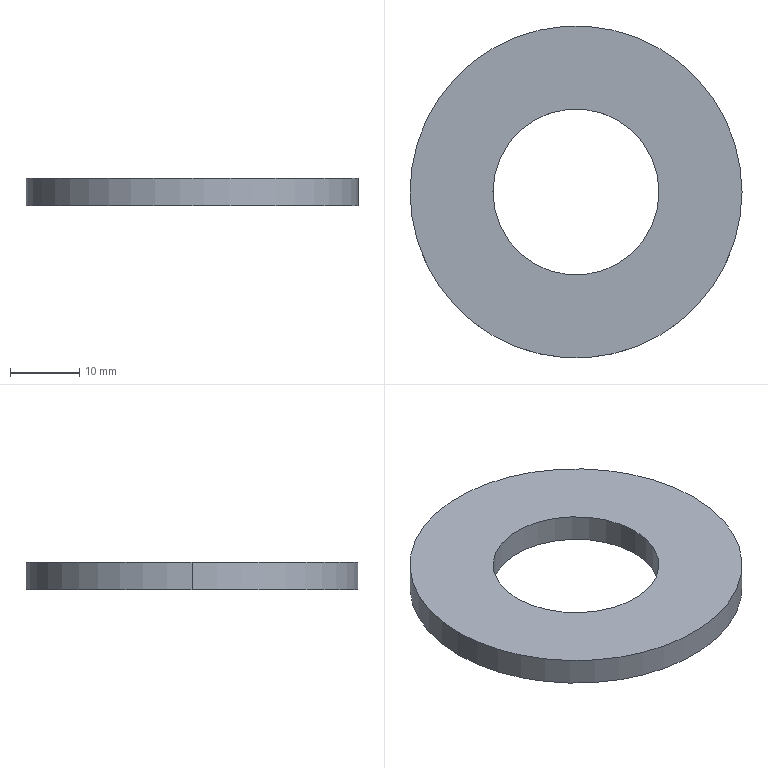Part | SolidWorks | features Extrusion 1 | 1 solid | 6 faces | box 48 x 48 x 4 mm | volume 5429 mm3 | cylinder 4 | plane 2 | commonest cylinder face diameters 24 x2 48 x2
STEP:
#1=CARTESIAN_POINT('',(-12.,0.,4.));
#2=VERTEX_POINT('',#1);
#3=CARTESIAN_POINT('',(12.,0.,4.));
#4=VERTEX_POINT('',#3);
#5=CARTESIAN_POINT('',(0.,0.,4.));
#6=DIRECTION('',(0.,0.,1.));
#7=DIRECTION('',(1.,0.,0.));
#8=AXIS2_PLACEMENT_3D('',#5,#6,#7);
#9=CIRCLE('',#8,12.);
#10=EDGE_CURVE('',#2,#4,#9,.T.);
#11=ORIENTED_EDGE('',*,*,#10,.T.);
#12=CARTESIAN_POINT('',(12.,0.,0.));
#13=VERTEX_POINT('',#12);
#14=CARTESIAN_POINT('',(12.,0.,4.));
#15=DIRECTION('',(0.,0.,-1.));
#16=VECTOR('',#15,1000.);
#17=LINE('',#14,#16);
#18=EDGE_CURVE('',#4,#13,#17,.T.);
#19=ORIENTED_EDGE('',*,*,#18,.T.);
#20=CARTESIAN_POINT('',(-12.,0.,0.));
#21=VERTEX_POINT('',#20);
#22=CARTESIAN_POINT('',(0.,0.,0.));
#23=DIRECTION('',(0.,0.,1.));
#24=DIRECTION('',(1.,0.,0.));
#25=AXIS2_PLACEMENT_3D('',#22,#23,#24);
#26=CIRCLE('',#25,12.);
#27=EDGE_CURVE('',#21,#13,#26,.T.);
#28=ORIENTED_EDGE('',*,*,#27,.F.);
#29=CARTESIAN_POINT('',(-12.,0.,4.));
#30=DIRECTION('',(0.,0.,-1.));
#31=VECTOR('',#30,1000.);
#32=LINE('',#29,#31);
#33=EDGE_CURVE('',#2,#21,#32,.T.);
#34=ORIENTED_EDGE('',*,*,#33,.F.);
#35=EDGE_LOOP('',(#11,#19,#28,#34));
#36=FACE_OUTER_BOUND('',#35,.T.);
#37=CARTESIAN_POINT('',(0.,0.,4.));
#38=DIRECTION('',(0.,0.,-1.));
#39=DIRECTION('',(-1.,0.,0.));
#40=AXIS2_PLACEMENT_3D('',#37,#38,#39);
#41=CYLINDRICAL_SURFACE('',#40,12.);
#42=ADVANCED_FACE('',(#36),#41,.F.);
#43=CARTESIAN_POINT('',(24.,0.,4.));
#44=VERTEX_POINT('',#43);
#45=CARTESIAN_POINT('',(-24.,0.,4.));
#46=VERTEX_POINT('',#45);
#47=CARTESIAN_POINT('',(0.,0.,4.));
#48=DIRECTION('',(0.,0.,1.));
#49=DIRECTION('',(1.,0.,0.));
#50=AXIS2_PLACEMENT_3D('',#47,#48,#49);
#51=CIRCLE('',#50,24.);
#52=EDGE_CURVE('',#44,#46,#51,.T.);
#53=ORIENTED_EDGE('',*,*,#52,.F.);
#54=CARTESIAN_POINT('',(24.,0.,0.));
#55=VERTEX_POINT('',#54);
#56=CARTESIAN_POINT('',(24.,0.,4.));
#57=DIRECTION('',(0.,0.,-1.));
#58=VECTOR('',#57,1000.);
#59=LINE('',#56,#58);
#60=EDGE_CURVE('',#44,#55,#59,.T.);
#61=ORIENTED_EDGE('',*,*,#60,.T.);
#62=CARTESIAN_POINT('',(-24.,0.,0.));
#63=VERTEX_POINT('',#62);
#64=CARTESIAN_POINT('',(0.,0.,0.));
#65=DIRECTION('',(0.,0.,1.));
#66=DIRECTION('',(1.,0.,0.));
#67=AXIS2_PLACEMENT_3D('',#64,#65,#66);
#68=CIRCLE('',#67,24.);
#69=EDGE_CURVE('',#55,#63,#68,.T.);
#70=ORIENTED_EDGE('',*,*,#69,.T.);
#71=CARTESIAN_POINT('',(-24.,0.,4.));
#72=DIRECTION('',(0.,0.,-1.));
#73=VECTOR('',#72,1000.);
#74=LINE('',#71,#73);
#75=EDGE_CURVE('',#46,#63,#74,.T.);
#76=ORIENTED_EDGE('',*,*,#75,.F.);
#77=EDGE_LOOP('',(#53,#61,#70,#76));
#78=FACE_OUTER_BOUND('',#77,.T.);
#79=CARTESIAN_POINT('',(0.,0.,4.));
#80=DIRECTION('',(0.,0.,-1.));
#81=DIRECTION('',(-1.,0.,0.));
#82=AXIS2_PLACEMENT_3D('',#79,#80,#81);
#83=CYLINDRICAL_SURFACE('',#82,24.);
#84=ADVANCED_FACE('',(#78),#83,.T.);
#85=CARTESIAN_POINT('',(0.,0.,4.));
#86=DIRECTION('',(0.,0.,1.));
#87=DIRECTION('',(1.,0.,0.));
#88=AXIS2_PLACEMENT_3D('',#85,#86,#87);
#89=CIRCLE('',#88,24.);
#90=EDGE_CURVE('',#46,#44,#89,.T.);
#91=ORIENTED_EDGE('',*,*,#90,.T.);
#92=ORIENTED_EDGE('',*,*,#52,.T.);
#93=EDGE_LOOP('',(#91,#92));
#94=FACE_OUTER_BOUND('',#93,.T.);
#95=ORIENTED_EDGE('',*,*,#10,.F.);
#96=CARTESIAN_POINT('',(0.,0.,4.));
#97=DIRECTION('',(0.,0.,1.));
#98=DIRECTION('',(1.,0.,0.));
#99=AXIS2_PLACEMENT_3D('',#96,#97,#98);
#100=CIRCLE('',#99,12.);
#101=EDGE_CURVE('',#4,#2,#100,.T.);
#102=ORIENTED_EDGE('',*,*,#101,.F.);
#103=EDGE_LOOP('',(#95,#102));
#104=FACE_BOUND('',#103,.T.);
#105=CARTESIAN_POINT('',(0.,0.,4.));
#106=DIRECTION('',(0.,0.,1.));
#107=DIRECTION('',(1.,0.,0.));
#108=AXIS2_PLACEMENT_3D('',#105,#106,#107);
#109=PLANE('',#108);
#110=ADVANCED_FACE('',(#94,#104),#109,.T.);
#111=CARTESIAN_POINT('',(0.,0.,0.));
#112=DIRECTION('',(0.,0.,1.));
#113=DIRECTION('',(1.,0.,0.));
#114=AXIS2_PLACEMENT_3D('',#111,#112,#113);
#115=CIRCLE('',#114,24.);
#116=EDGE_CURVE('',#63,#55,#115,.T.);
#117=ORIENTED_EDGE('',*,*,#116,.F.);
#118=ORIENTED_EDGE('',*,*,#69,.F.);
#119=EDGE_LOOP('',(#117,#118));
#120=FACE_OUTER_BOUND('',#119,.T.);
#121=ORIENTED_EDGE('',*,*,#27,.T.);
#122=CARTESIAN_POINT('',(0.,0.,0.));
#123=DIRECTION('',(0.,0.,1.));
#124=DIRECTION('',(1.,0.,0.));
#125=AXIS2_PLACEMENT_3D('',#122,#123,#124);
#126=CIRCLE('',#125,12.);
#127=EDGE_CURVE('',#13,#21,#126,.T.);
#128=ORIENTED_EDGE('',*,*,#127,.T.);
#129=EDGE_LOOP('',(#121,#128));
#130=FACE_BOUND('',#129,.T.);
#131=CARTESIAN_POINT('',(0.,0.,0.));
#132=DIRECTION('',(0.,0.,1.));
#133=DIRECTION('',(1.,0.,0.));
#134=AXIS2_PLACEMENT_3D('',#131,#132,#133);
#135=PLANE('',#134);
#136=ADVANCED_FACE('',(#120,#130),#135,.F.);
#137=ORIENTED_EDGE('',*,*,#60,.F.);
#138=ORIENTED_EDGE('',*,*,#90,.F.);
#139=ORIENTED_EDGE('',*,*,#75,.T.);
#140=ORIENTED_EDGE('',*,*,#116,.T.);
#141=EDGE_LOOP('',(#137,#138,#139,#140));
#142=FACE_OUTER_BOUND('',#141,.T.);
#143=CARTESIAN_POINT('',(0.,0.,4.));
#144=DIRECTION('',(0.,0.,-1.));
#145=DIRECTION('',(-1.,0.,0.));
#146=AXIS2_PLACEMENT_3D('',#143,#144,#145);
#147=CYLINDRICAL_SURFACE('',#146,24.);
#148=ADVANCED_FACE('',(#142),#147,.T.);
#149=ORIENTED_EDGE('',*,*,#18,.F.);
#150=ORIENTED_EDGE('',*,*,#101,.T.);
#151=ORIENTED_EDGE('',*,*,#33,.T.);
#152=ORIENTED_EDGE('',*,*,#127,.F.);
#153=EDGE_LOOP('',(#149,#150,#151,#152));
#154=FACE_OUTER_BOUND('',#153,.T.);
#155=CARTESIAN_POINT('',(0.,0.,4.));
#156=DIRECTION('',(0.,0.,-1.));
#157=DIRECTION('',(-1.,0.,0.));
#158=AXIS2_PLACEMENT_3D('',#155,#156,#157);
#159=CYLINDRICAL_SURFACE('',#158,12.);
#160=ADVANCED_FACE('',(#154),#159,.F.);
#161=CLOSED_SHELL('',(#42,#84,#110,#136,#148,#160));
#162=MANIFOLD_SOLID_BREP('',#161);
#163=CARTESIAN_POINT('',(0.,0.,0.));
#164=DIRECTION('',(0.,0.,1.));
#165=DIRECTION('',(1.,0.,0.));
#166=AXIS2_PLACEMENT_3D('',#163,#164,#165);
#167=(LENGTH_UNIT()NAMED_UNIT(*)SI_UNIT(.MILLI.,.METRE.));
#168=UNCERTAINTY_MEASURE_WITH_UNIT(LENGTH_MEASURE(0.00001),#167,'','');
#169=(NAMED_UNIT(*)PLANE_ANGLE_UNIT()SI_UNIT($,.RADIAN.));
#170=(NAMED_UNIT(*)SI_UNIT($,.STERADIAN.)SOLID_ANGLE_UNIT());
#171=(GEOMETRIC_REPRESENTATION_CONTEXT(3)GLOBAL_UNCERTAINTY_ASSIGNED_CONTEXT((#168))GLOBAL_UNIT_ASSIGNED_CONTEXT((#167,#169,#170))REPRESENTATION_CONTEXT('',''));
#172=ADVANCED_BREP_SHAPE_REPRESENTATION('',(#162,#166),#171);